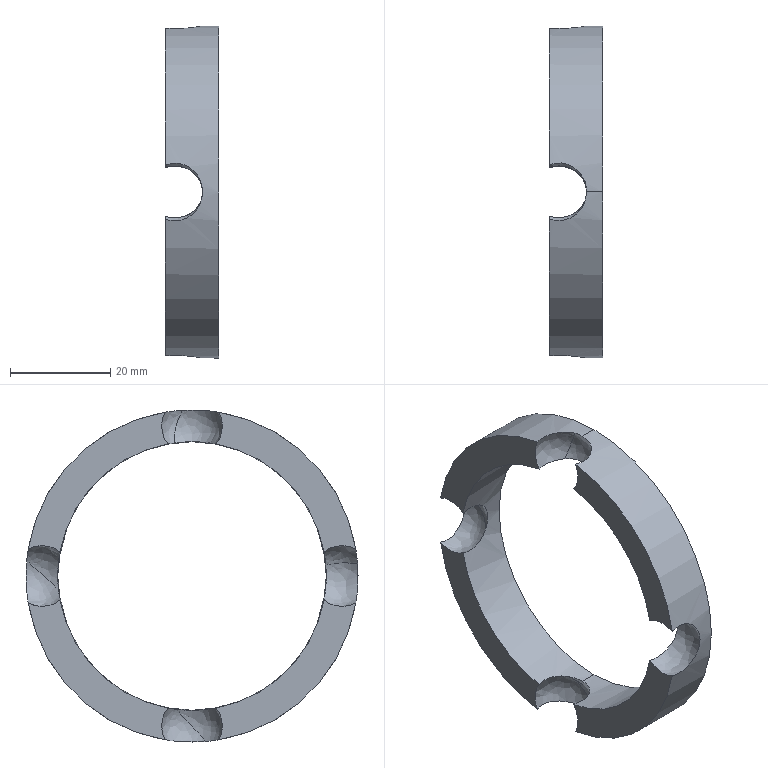Part | SolidWorks | features BaseBody 1 | 1 solid | 17 faces | volume 10638 mm3 | spline 10 | plane 5 | cylinder 2 | commonest cylinder face diameters 66.35 x2
STEP:
#1=CARTESIAN_POINT('',(4.998,48.263,51.37));
#2=VERTEX_POINT('',#1);
#3=CARTESIAN_POINT('',(-1.905,48.619,54.059));
#4=VERTEX_POINT('',#3);
#5=CARTESIAN_POINT('',(4.998,48.263,51.37));
#6=CARTESIAN_POINT('',(4.85,48.288,51.674));
#7=CARTESIAN_POINT('',(4.671,48.316,51.963));
#8=CARTESIAN_POINT('',(4.265,48.377,52.495));
#9=CARTESIAN_POINT('',(4.034,48.409,52.744));
#10=CARTESIAN_POINT('',(3.53,48.473,53.191));
#11=CARTESIAN_POINT('',(3.259,48.504,53.389));
#12=CARTESIAN_POINT('',(2.684,48.561,53.735));
#13=CARTESIAN_POINT('',(2.377,48.587,53.884));
#14=CARTESIAN_POINT('',(1.748,48.63,54.121));
#15=CARTESIAN_POINT('',(1.425,48.647,54.212));
#16=CARTESIAN_POINT('',(0.7618,48.671,54.337));
#17=CARTESIAN_POINT('',(0.4216,48.678,54.371));
#18=CARTESIAN_POINT('',(-0.5983,48.681,54.386));
#19=CARTESIAN_POINT('',(-1.263,48.66,54.281));
#20=CARTESIAN_POINT('',(-1.905,48.619,54.059));
#21=B_SPLINE_CURVE_WITH_KNOTS('',3,(#5,#6,#7,#8,#9,#10,#11,#12,#13,#14,#15,#16,#17,#18,#19,#20),.UNSPECIFIED.,.F.,.F.,(4,2,2,2,2,2,2,4),(0.01061,0.01162,0.01262,0.01363,0.01463,0.01564,0.01665,0.01866),.UNSPECIFIED.);
#22=EDGE_CURVE('',#2,#4,#21,.T.);
#23=ORIENTED_EDGE('',*,*,#22,.F.);
#24=CARTESIAN_POINT('',(5.424,47.273,51.598));
#25=VERTEX_POINT('',#24);
#26=CARTESIAN_POINT('',(0.,45.,49.2));
#27=DIRECTION('',(0.4147,-0.03029,-0.9094));
#28=DIRECTION('',(-0.854,-0.3579,-0.3775));
#29=AXIS2_PLACEMENT_3D('',#26,#27,#28);
#30=CIRCLE('',#29,6.351);
#31=EDGE_CURVE('',#2,#25,#30,.T.);
#32=ORIENTED_EDGE('',*,*,#31,.T.);
#33=CARTESIAN_POINT('',(5.009,41.911,51.587));
#34=VERTEX_POINT('',#33);
#35=CARTESIAN_POINT('',(0.,45.,49.2));
#36=DIRECTION('',(-0.4147,0.03029,0.9094));
#37=DIRECTION('',(-0.854,-0.3579,-0.3775));
#38=AXIS2_PLACEMENT_3D('',#35,#36,#37);
#39=CIRCLE('',#38,6.351);
#40=EDGE_CURVE('',#34,#25,#39,.T.);
#41=ORIENTED_EDGE('',*,*,#40,.F.);
#42=CARTESIAN_POINT('',(-1.905,42.269,54.608));
#43=VERTEX_POINT('',#42);
#44=CARTESIAN_POINT('',(-1.905,42.269,54.608));
#45=CARTESIAN_POINT('',(-1.577,42.29,54.734));
#46=CARTESIAN_POINT('',(-1.243,42.305,54.826));
#47=CARTESIAN_POINT('',(-0.7316,42.321,54.914));
#48=CARTESIAN_POINT('',(-0.5596,42.325,54.935));
#49=CARTESIAN_POINT('',(-0.2125,42.329,54.961));
#50=CARTESIAN_POINT('',(-0.03628,42.33,54.965));
#51=CARTESIAN_POINT('',(0.4893,42.327,54.951));
#52=CARTESIAN_POINT('',(0.8336,42.32,54.908));
#53=CARTESIAN_POINT('',(1.511,42.293,54.754));
#54=CARTESIAN_POINT('',(1.847,42.274,54.642));
#55=CARTESIAN_POINT('',(2.481,42.228,54.359));
#56=CARTESIAN_POINT('',(2.782,42.202,54.188));
#57=CARTESIAN_POINT('',(3.21,42.158,53.889));
#58=CARTESIAN_POINT('',(3.349,42.143,53.781));
#59=CARTESIAN_POINT('',(3.614,42.112,53.555));
#60=CARTESIAN_POINT('',(3.74,42.096,53.436));
#61=CARTESIAN_POINT('',(4.102,42.05,53.064));
#62=CARTESIAN_POINT('',(4.319,42.019,52.794));
#63=CARTESIAN_POINT('',(4.707,41.961,52.211));
#64=CARTESIAN_POINT('',(4.872,41.934,51.905));
#65=CARTESIAN_POINT('',(5.009,41.911,51.587));
#66=B_SPLINE_CURVE_WITH_KNOTS('',3,(#44,#45,#46,#47,#48,#49,#50,#51,#52,#53,#54,#55,#56,#57,#58,#59,#60,#61,#62,#63,#64,#65),.UNSPECIFIED.,.F.,.F.,(4,2,2,2,2,2,2,2,2,2,4),(-0.01955,-0.01851,-0.01799,-0.01747,-0.01643,-0.0154,-0.01436,-0.01384,-0.01332,-0.01228,-0.01124),.UNSPECIFIED.);
#67=EDGE_CURVE('',#43,#34,#66,.T.);
#68=ORIENTED_EDGE('',*,*,#67,.F.);
#69=CARTESIAN_POINT('',(-1.905,45.,49.2));
#70=DIRECTION('',(1.,0.,0.));
#71=DIRECTION('',(0.,0.,-1.));
#72=AXIS2_PLACEMENT_3D('',#69,#70,#71);
#73=CIRCLE('',#72,6.059);
#74=EDGE_CURVE('',#4,#43,#73,.T.);
#75=ORIENTED_EDGE('',*,*,#74,.F.);
#76=EDGE_LOOP('',(#23,#32,#41,#68,#75));
#77=FACE_OUTER_BOUND('',#76,.T.);
#78=CARTESIAN_POINT('',(-2.519,50.674,47.862));
#79=CARTESIAN_POINT('',(-7.762,51.057,59.358));
#80=CARTESIAN_POINT('',(-3.792,39.261,61.561));
#81=CARTESIAN_POINT('',(1.451,38.878,50.065));
#82=CARTESIAN_POINT('',(0.7712,52.475,49.303));
#83=CARTESIAN_POINT('',(-4.799,52.882,61.518));
#84=CARTESIAN_POINT('',(-0.5807,40.346,63.86));
#85=CARTESIAN_POINT('',(4.99,39.939,51.644));
#86=CARTESIAN_POINT('',(4.162,51.023,50.897));
#87=CARTESIAN_POINT('',(0.8289,51.267,58.206));
#88=CARTESIAN_POINT('',(3.353,43.767,59.607));
#89=CARTESIAN_POINT('',(6.686,43.523,52.298));
#90=CARTESIAN_POINT('',(5.424,47.273,51.598));
#91=CARTESIAN_POINT('',(5.424,47.273,51.598));
#92=CARTESIAN_POINT('',(5.424,47.273,51.598));
#93=CARTESIAN_POINT('',(5.424,47.273,51.598));
#94=(BOUNDED_SURFACE()B_SPLINE_SURFACE(3,3,((#78,#79,#80,#81),(#82,#83,#84,#85),(#86,#87,#88,#89),(#90,#91,#92,#93)),.UNSPECIFIED.,.F.,.F.,.F.)B_SPLINE_SURFACE_WITH_KNOTS((4,4),(4,4),(0.,1.),(0.,1.),.UNSPECIFIED.)GEOMETRIC_REPRESENTATION_ITEM()RATIONAL_B_SPLINE_SURFACE(((1.,0.3333,0.3333,1.),(0.7809,0.2603,0.2603,0.7809),(0.7809,0.2603,0.2603,0.7809),(1.,0.3333,0.3333,1.)))REPRESENTATION_ITEM('')SURFACE());
#95=ADVANCED_FACE('',(#77),#94,.T.);
#96=CARTESIAN_POINT('',(4.024,78.538,75.791));
#97=VERTEX_POINT('',#96);
#98=CARTESIAN_POINT('',(-1.905,79.859,75.581));
#99=VERTEX_POINT('',#98);
#100=CARTESIAN_POINT('',(4.024,78.538,75.791));
#101=CARTESIAN_POINT('',(3.838,78.726,75.766));
#102=CARTESIAN_POINT('',(3.637,78.9,75.741));
#103=CARTESIAN_POINT('',(3.21,79.218,75.692));
#104=CARTESIAN_POINT('',(2.983,79.363,75.668));
#105=CARTESIAN_POINT('',(2.515,79.615,75.625));
#106=CARTESIAN_POINT('',(2.273,79.724,75.606));
#107=CARTESIAN_POINT('',(1.774,79.909,75.572));
#108=CARTESIAN_POINT('',(1.515,79.985,75.558));
#109=CARTESIAN_POINT('',(0.9921,80.099,75.536));
#110=CARTESIAN_POINT('',(0.7281,80.138,75.528));
#111=CARTESIAN_POINT('',(0.1951,80.18,75.52));
#112=CARTESIAN_POINT('',(-0.07553,80.182,75.52));
#113=CARTESIAN_POINT('',(-0.8755,80.136,75.529));
#114=CARTESIAN_POINT('',(-1.397,80.034,75.549));
#115=CARTESIAN_POINT('',(-1.905,79.859,75.581));
#116=B_SPLINE_CURVE_WITH_KNOTS('',3,(#100,#101,#102,#103,#104,#105,#106,#107,#108,#109,#110,#111,#112,#113,#114,#115),.UNSPECIFIED.,.F.,.F.,(4,2,2,2,2,2,2,4),(0.00392,0.004717,0.005515,0.006312,0.007109,0.007906,0.008703,0.0103),.UNSPECIFIED.);
#117=EDGE_CURVE('',#97,#99,#116,.T.);
#118=ORIENTED_EDGE('',*,*,#117,.F.);
#119=CARTESIAN_POINT('',(5.424,77.273,81.598));
#120=VERTEX_POINT('',#119);
#121=CARTESIAN_POINT('',(0.,75.,79.2));
#122=DIRECTION('',(0.4774,-0.8276,-0.2953));
#123=DIRECTION('',(-0.854,-0.3579,-0.3775));
#124=AXIS2_PLACEMENT_3D('',#121,#122,#123);
#125=CIRCLE('',#124,6.351);
#126=EDGE_CURVE('',#97,#120,#125,.T.);
#127=ORIENTED_EDGE('',*,*,#126,.T.);
#128=CARTESIAN_POINT('',(5.2,76.886,82.321));
#129=VERTEX_POINT('',#128);
#130=CARTESIAN_POINT('',(0.,75.,79.2));
#131=DIRECTION('',(-0.4774,0.8276,0.2953));
#132=DIRECTION('',(-0.854,-0.3579,-0.3775));
#133=AXIS2_PLACEMENT_3D('',#130,#131,#132);
#134=CIRCLE('',#133,6.351);
#135=EDGE_CURVE('',#129,#120,#134,.T.);
#136=ORIENTED_EDGE('',*,*,#135,.F.);
#137=CARTESIAN_POINT('',(-1.905,80.408,81.931));
#138=VERTEX_POINT('',#137);
#139=CARTESIAN_POINT('',(-1.905,80.408,81.931));
#140=CARTESIAN_POINT('',(-1.556,80.542,81.909));
#141=CARTESIAN_POINT('',(-1.2,80.638,81.893));
#142=CARTESIAN_POINT('',(-0.6542,80.725,81.877));
#143=CARTESIAN_POINT('',(-0.4706,80.744,81.874));
#144=CARTESIAN_POINT('',(-0.09979,80.764,81.87));
#145=CARTESIAN_POINT('',(0.08844,80.765,81.87));
#146=CARTESIAN_POINT('',(0.6454,80.736,81.875));
#147=CARTESIAN_POINT('',(1.01,80.678,81.886));
#148=CARTESIAN_POINT('',(1.726,80.487,81.918));
#149=CARTESIAN_POINT('',(2.077,80.352,81.941));
#150=CARTESIAN_POINT('',(2.735,80.019,81.994));
#151=CARTESIAN_POINT('',(3.046,79.819,82.024));
#152=CARTESIAN_POINT('',(3.629,79.354,82.089));
#153=CARTESIAN_POINT('',(3.892,79.096,82.122));
#154=CARTESIAN_POINT('',(4.367,78.532,82.188));
#155=CARTESIAN_POINT('',(4.579,78.223,82.22));
#156=CARTESIAN_POINT('',(4.937,77.576,82.276));
#157=CARTESIAN_POINT('',(5.084,77.238,82.301));
#158=CARTESIAN_POINT('',(5.2,76.886,82.321));
#159=B_SPLINE_CURVE_WITH_KNOTS('',3,(#139,#140,#141,#142,#143,#144,#145,#146,#147,#148,#149,#150,#151,#152,#153,#154,#155,#156,#157,#158),.UNSPECIFIED.,.F.,.F.,(4,2,2,2,2,2,2,2,2,4),(-0.01954,-0.01843,-0.01788,-0.01733,-0.01622,-0.01512,-0.01402,-0.01291,-0.01181,-0.0107),.UNSPECIFIED.);
#160=EDGE_CURVE('',#138,#129,#159,.T.);
#161=ORIENTED_EDGE('',*,*,#160,.F.);
#162=CARTESIAN_POINT('',(-1.905,75.,79.2));
#163=DIRECTION('',(1.,0.,0.));
#164=DIRECTION('',(0.,0.,-1.));
#165=AXIS2_PLACEMENT_3D('',#162,#163,#164);
#166=CIRCLE('',#165,6.059);
#167=EDGE_CURVE('',#99,#138,#166,.T.);
#168=ORIENTED_EDGE('',*,*,#167,.F.);
#169=EDGE_LOOP('',(#118,#127,#136,#161,#168));
#170=FACE_OUTER_BOUND('',#169,.T.);
#171=CARTESIAN_POINT('',(0.1572,77.214,73.249));
#172=CARTESIAN_POINT('',(-5.774,87.496,76.918));
#173=CARTESIAN_POINT('',(-8.343,82.124,87.823));
#174=CARTESIAN_POINT('',(-2.412,71.841,84.154));
#175=CARTESIAN_POINT('',(3.996,79.137,74.066));
#176=CARTESIAN_POINT('',(-2.803,90.923,78.271));
#177=CARTESIAN_POINT('',(-5.747,84.765,90.77));
#178=CARTESIAN_POINT('',(1.051,72.979,86.565));
#179=CARTESIAN_POINT('',(6.327,79.163,77.762));
#180=CARTESIAN_POINT('',(2.155,86.396,80.343));
#181=CARTESIAN_POINT('',(0.3478,82.617,88.014));
#182=CARTESIAN_POINT('',(4.52,75.384,85.433));
#183=CARTESIAN_POINT('',(5.424,77.273,81.598));
#184=CARTESIAN_POINT('',(5.424,77.273,81.598));
#185=CARTESIAN_POINT('',(5.424,77.273,81.598));
#186=CARTESIAN_POINT('',(5.424,77.273,81.598));
#187=(BOUNDED_SURFACE()B_SPLINE_SURFACE(3,3,((#171,#172,#173,#174),(#175,#176,#177,#178),(#179,#180,#181,#182),(#183,#184,#185,#186)),.UNSPECIFIED.,.F.,.F.,.T.)B_SPLINE_SURFACE_WITH_KNOTS((4,4),(4,4),(0.,1.),(0.,1.),.UNSPECIFIED.)GEOMETRIC_REPRESENTATION_ITEM()RATIONAL_B_SPLINE_SURFACE(((1.,0.3333,0.3333,1.),(0.7529,0.251,0.251,0.7529),(0.7529,0.251,0.251,0.7529),(1.,0.3333,0.3333,1.)))REPRESENTATION_ITEM('')SURFACE());
#188=ADVANCED_FACE('',(#170),#187,.T.);
#189=CARTESIAN_POINT('',(4.675,101.685,46.463));
#190=VERTEX_POINT('',#189);
#191=CARTESIAN_POINT('',(-1.905,101.381,44.341));
#192=VERTEX_POINT('',#191);
#193=CARTESIAN_POINT('',(4.675,101.685,46.463));
#194=CARTESIAN_POINT('',(4.505,101.659,46.205));
#195=CARTESIAN_POINT('',(4.314,101.63,45.964));
#196=CARTESIAN_POINT('',(3.887,101.572,45.516));
#197=CARTESIAN_POINT('',(3.652,101.542,45.309));
#198=CARTESIAN_POINT('',(3.156,101.486,44.943));
#199=CARTESIAN_POINT('',(2.894,101.459,44.782));
#200=CARTESIAN_POINT('',(2.339,101.411,44.501));
#201=CARTESIAN_POINT('',(2.05,101.389,44.384));
#202=CARTESIAN_POINT('',(1.462,101.355,44.199));
#203=CARTESIAN_POINT('',(1.16,101.342,44.13));
#204=CARTESIAN_POINT('',(0.5433,101.324,44.04));
#205=CARTESIAN_POINT('',(0.2296,101.32,44.019));
#206=CARTESIAN_POINT('',(-0.7067,101.323,44.033));
#207=CARTESIAN_POINT('',(-1.314,101.344,44.137));
#208=CARTESIAN_POINT('',(-1.905,101.381,44.341));
#209=B_SPLINE_CURVE_WITH_KNOTS('',3,(#193,#194,#195,#196,#197,#198,#199,#200,#201,#202,#203,#204,#205,#206,#207,#208),.UNSPECIFIED.,.F.,.F.,(4,2,2,2,2,2,2,4),(0.01126,0.01218,0.01311,0.01403,0.01496,0.01588,0.01681,0.01866),.UNSPECIFIED.);
#210=EDGE_CURVE('',#190,#192,#209,.T.);
#211=ORIENTED_EDGE('',*,*,#210,.F.);
#212=CARTESIAN_POINT('',(5.424,107.273,51.598));
#213=VERTEX_POINT('',#212);
#214=CARTESIAN_POINT('',(0.,105.,49.2));
#215=DIRECTION('',(-0.0446,-0.6727,0.7386));
#216=DIRECTION('',(-0.854,-0.3579,-0.3775));
#217=AXIS2_PLACEMENT_3D('',#214,#215,#216);
#218=CIRCLE('',#217,6.351);
#219=EDGE_CURVE('',#190,#213,#218,.T.);
#220=ORIENTED_EDGE('',*,*,#219,.T.);
#221=CARTESIAN_POINT('',(4.674,108.035,52.246));
#222=VERTEX_POINT('',#221);
#223=CARTESIAN_POINT('',(0.,105.,49.2));
#224=DIRECTION('',(0.0446,0.6727,-0.7386));
#225=DIRECTION('',(-0.854,-0.3579,-0.3775));
#226=AXIS2_PLACEMENT_3D('',#223,#224,#225);
#227=CIRCLE('',#226,6.351);
#228=EDGE_CURVE('',#222,#213,#227,.T.);
#229=ORIENTED_EDGE('',*,*,#228,.F.);
#230=CARTESIAN_POINT('',(-1.905,107.731,43.792));
#231=VERTEX_POINT('',#230);
#232=CARTESIAN_POINT('',(-1.905,107.731,43.792));
#233=CARTESIAN_POINT('',(-1.355,107.696,43.581));
#234=CARTESIAN_POINT('',(-0.7877,107.675,43.464));
#235=CARTESIAN_POINT('',(0.09096,107.669,43.431));
#236=CARTESIAN_POINT('',(0.3863,107.672,43.444));
#237=CARTESIAN_POINT('',(0.9633,107.685,43.518));
#238=CARTESIAN_POINT('',(1.248,107.695,43.579));
#239=CARTESIAN_POINT('',(1.808,107.724,43.747));
#240=CARTESIAN_POINT('',(2.083,107.742,43.856));
#241=CARTESIAN_POINT('',(2.605,107.783,44.111));
#242=CARTESIAN_POINT('',(2.854,107.806,44.26));
#243=CARTESIAN_POINT('',(3.33,107.855,44.597));
#244=CARTESIAN_POINT('',(3.556,107.881,44.787));
#245=CARTESIAN_POINT('',(3.97,107.933,45.193));
#246=CARTESIAN_POINT('',(4.161,107.959,45.412));
#247=CARTESIAN_POINT('',(4.509,108.009,45.879));
#248=CARTESIAN_POINT('',(4.667,108.033,46.128));
#249=CARTESIAN_POINT('',(4.94,108.077,46.642));
#250=CARTESIAN_POINT('',(5.057,108.097,46.907));
#251=CARTESIAN_POINT('',(5.252,108.13,47.456));
#252=CARTESIAN_POINT('',(5.33,108.144,47.742));
#253=CARTESIAN_POINT('',(5.443,108.164,48.315));
#254=CARTESIAN_POINT('',(5.478,108.171,48.603));
#255=CARTESIAN_POINT('',(5.507,108.176,49.184));
#256=CARTESIAN_POINT('',(5.501,108.175,49.478));
#257=CARTESIAN_POINT('',(5.446,108.165,50.063));
#258=CARTESIAN_POINT('',(5.398,108.156,50.35));
#259=CARTESIAN_POINT('',(5.261,108.132,50.914));
#260=CARTESIAN_POINT('',(5.172,108.116,51.191));
#261=CARTESIAN_POINT('',(4.952,108.079,51.734));
#262=CARTESIAN_POINT('',(4.822,108.058,51.997));
#263=CARTESIAN_POINT('',(4.674,108.035,52.246));
#264=B_SPLINE_CURVE_WITH_KNOTS('',3,(#232,#233,#234,#235,#236,#237,#238,#239,#240,#241,#242,#243,#244,#245,#246,#247,#248,#249,#250,#251,#252,#253,#254,#255,#256,#257,#258,#259,#260,#261,#262,#263),.UNSPECIFIED.,.F.,.F.,(4,2,2,2,2,2,2,2,2,2,2,2,2,2,2,4),(0.,0.001739,0.002609,0.003479,0.004349,0.005218,0.006088,0.006958,0.007827,0.008697,0.009567,0.01044,0.01131,0.01218,0.01305,0.01392),.UNSPECIFIED.);
#265=EDGE_CURVE('',#231,#222,#264,.T.);
#266=ORIENTED_EDGE('',*,*,#265,.F.);
#267=CARTESIAN_POINT('',(-1.905,105.,49.2));
#268=DIRECTION('',(1.,0.,0.));
#269=DIRECTION('',(0.,0.,-1.));
#270=AXIS2_PLACEMENT_3D('',#267,#268,#269);
#271=CIRCLE('',#270,6.059);
#272=EDGE_CURVE('',#192,#231,#271,.T.);
#273=ORIENTED_EDGE('',*,*,#272,.F.);
#274=EDGE_LOOP('',(#211,#220,#229,#266,#273));
#275=FACE_OUTER_BOUND('',#274,.T.);
#276=CARTESIAN_POINT('',(-1.969,100.595,45.07));
#277=CARTESIAN_POINT('',(-1.6,106.163,38.956));
#278=CARTESIAN_POINT('',(-5.89,111.524,43.579));
#279=CARTESIAN_POINT('',(-6.259,105.956,49.693));
#280=CARTESIAN_POINT('',(4.705,98.783,43.822));
#281=CARTESIAN_POINT('',(5.549,111.521,29.835));
#282=CARTESIAN_POINT('',(-4.266,123.785,40.411));
#283=CARTESIAN_POINT('',(-5.111,111.047,54.398));
#284=CARTESIAN_POINT('',(9.066,102.722,47.673));
#285=CARTESIAN_POINT('',(9.693,112.176,37.293));
#286=CARTESIAN_POINT('',(2.409,121.277,45.142));
#287=CARTESIAN_POINT('',(1.782,111.824,55.522));
#288=CARTESIAN_POINT('',(5.424,107.273,51.598));
#289=CARTESIAN_POINT('',(5.424,107.273,51.598));
#290=CARTESIAN_POINT('',(5.424,107.273,51.598));
#291=CARTESIAN_POINT('',(5.424,107.273,51.598));
#292=(BOUNDED_SURFACE()B_SPLINE_SURFACE(3,3,((#276,#277,#278,#279),(#280,#281,#282,#283),(#284,#285,#286,#287),(#288,#289,#290,#291)),.UNSPECIFIED.,.F.,.F.,.F.)B_SPLINE_SURFACE_WITH_KNOTS((4,4),(4,4),(0.,1.),(0.,1.),.UNSPECIFIED.)GEOMETRIC_REPRESENTATION_ITEM()RATIONAL_B_SPLINE_SURFACE(((1.,0.3333,0.3333,1.),(0.565,0.1883,0.1883,0.565),(0.565,0.1883,0.1883,0.565),(1.,0.3333,0.3333,1.)))REPRESENTATION_ITEM('')SURFACE());
#293=ADVANCED_FACE('',(#275),#292,.T.);
#294=CARTESIAN_POINT('',(4.358,78.168,22.563));
#295=VERTEX_POINT('',#294);
#296=CARTESIAN_POINT('',(5.5,75.,22.375));
#297=VERTEX_POINT('',#296);
#298=CARTESIAN_POINT('',(4.358,78.168,22.563));
#299=CARTESIAN_POINT('',(4.537,77.949,22.537));
#300=CARTESIAN_POINT('',(4.7,77.713,22.511));
#301=CARTESIAN_POINT('',(4.985,77.214,22.465));
#302=CARTESIAN_POINT('',(5.105,76.956,22.445));
#303=CARTESIAN_POINT('',(5.396,76.155,22.395));
#304=CARTESIAN_POINT('',(5.5,75.579,22.375));
#305=CARTESIAN_POINT('',(5.5,75.,22.375));
#306=B_SPLINE_CURVE_WITH_KNOTS('',3,(#298,#299,#300,#301,#302,#303,#304,#305),.UNSPECIFIED.,.F.,.F.,(4,2,2,4),(0.004949,0.005803,0.006658,0.008367),.UNSPECIFIED.);
#307=EDGE_CURVE('',#295,#297,#306,.T.);
#308=ORIENTED_EDGE('',*,*,#307,.F.);
#309=CARTESIAN_POINT('',(5.424,77.273,21.598));
#310=VERTEX_POINT('',#309);
#311=CARTESIAN_POINT('',(0.,75.,19.2));
#312=DIRECTION('',(-0.004434,0.7307,-0.6827));
#313=DIRECTION('',(-0.854,-0.3579,-0.3775));
#314=AXIS2_PLACEMENT_3D('',#311,#312,#313);
#315=CIRCLE('',#314,6.351);
#316=EDGE_CURVE('',#295,#310,#315,.T.);
#317=ORIENTED_EDGE('',*,*,#316,.T.);
#318=CARTESIAN_POINT('',(4.798,72.175,16.145));
#319=VERTEX_POINT('',#318);
#320=CARTESIAN_POINT('',(0.,75.,19.2));
#321=DIRECTION('',(0.004434,-0.7307,0.6827));
#322=DIRECTION('',(-0.854,-0.3579,-0.3775));
#323=AXIS2_PLACEMENT_3D('',#320,#321,#322);
#324=CIRCLE('',#323,6.351);
#325=EDGE_CURVE('',#319,#310,#324,.T.);
#326=ORIENTED_EDGE('',*,*,#325,.F.);
#327=CARTESIAN_POINT('',(-1.905,69.592,16.469));
#328=VERTEX_POINT('',#327);
#329=CARTESIAN_POINT('',(-1.905,69.592,16.469));
#330=CARTESIAN_POINT('',(-1.288,69.355,16.508));
#331=CARTESIAN_POINT('',(-0.6467,69.236,16.53));
#332=CARTESIAN_POINT('',(0.347,69.239,16.529));
#333=CARTESIAN_POINT('',(0.6729,69.271,16.523));
#334=CARTESIAN_POINT('',(1.314,69.393,16.502));
#335=CARTESIAN_POINT('',(1.632,69.485,16.486));
#336=CARTESIAN_POINT('',(2.245,69.725,16.447));
#337=CARTESIAN_POINT('',(2.536,69.872,16.423));
#338=CARTESIAN_POINT('',(3.091,70.216,16.371));
#339=CARTESIAN_POINT('',(3.356,70.416,16.343));
#340=CARTESIAN_POINT('',(3.841,70.854,16.284));
#341=CARTESIAN_POINT('',(4.062,71.093,16.255));
#342=CARTESIAN_POINT('',(4.464,71.608,16.198));
#343=CARTESIAN_POINT('',(4.645,71.887,16.17));
#344=CARTESIAN_POINT('',(4.798,72.175,16.145));
#345=B_SPLINE_CURVE_WITH_KNOTS('',3,(#329,#330,#331,#332,#333,#334,#335,#336,#337,#338,#339,#340,#341,#342,#343,#344),.UNSPECIFIED.,.F.,.F.,(4,2,2,2,2,2,2,4),(-0.001944,0.00001557,0.0009952,0.001975,0.002955,0.003934,0.004914,0.005894),.UNSPECIFIED.);
#346=EDGE_CURVE('',#328,#319,#345,.T.);
#347=ORIENTED_EDGE('',*,*,#346,.F.);
#348=CARTESIAN_POINT('',(-1.905,70.141,22.819));
#349=VERTEX_POINT('',#348);
#350=CARTESIAN_POINT('',(-1.905,75.,19.2));
#351=DIRECTION('',(1.,0.,0.));
#352=DIRECTION('',(0.,0.,-1.));
#353=AXIS2_PLACEMENT_3D('',#350,#351,#352);
#354=CIRCLE('',#353,6.059);
#355=EDGE_CURVE('',#349,#328,#354,.T.);
#356=ORIENTED_EDGE('',*,*,#355,.F.);
#357=CARTESIAN_POINT('',(5.5,75.,22.375));
#358=CARTESIAN_POINT('',(5.5,74.564,22.375));
#359=CARTESIAN_POINT('',(5.443,74.139,22.386));
#360=CARTESIAN_POINT('',(5.276,73.515,22.415));
#361=CARTESIAN_POINT('',(5.206,73.308,22.428));
#362=CARTESIAN_POINT('',(5.041,72.91,22.456));
#363=CARTESIAN_POINT('',(4.947,72.718,22.472));
#364=CARTESIAN_POINT('',(4.627,72.16,22.523));
#365=CARTESIAN_POINT('',(4.364,71.811,22.563));
#366=CARTESIAN_POINT('',(3.916,71.35,22.624));
#367=CARTESIAN_POINT('',(3.758,71.206,22.644));
#368=CARTESIAN_POINT('',(3.425,70.936,22.684));
#369=CARTESIAN_POINT('',(3.249,70.811,22.704));
#370=CARTESIAN_POINT('',(2.7,70.466,22.76));
#371=CARTESIAN_POINT('',(2.313,70.282,22.793));
#372=CARTESIAN_POINT('',(1.703,70.071,22.832));
#373=CARTESIAN_POINT('',(1.493,70.012,22.843));
#374=CARTESIAN_POINT('',(1.071,69.917,22.861));
#375=CARTESIAN_POINT('',(0.8587,69.882,22.868));
#376=CARTESIAN_POINT('',(0.2161,69.811,22.882));
#377=CARTESIAN_POINT('',(-0.2224,69.812,22.881));
#378=CARTESIAN_POINT('',(-1.076,69.906,22.863));
#379=CARTESIAN_POINT('',(-1.495,69.999,22.845));
#380=CARTESIAN_POINT('',(-1.905,70.141,22.819));
#381=B_SPLINE_CURVE_WITH_KNOTS('',3,(#357,#358,#359,#360,#361,#362,#363,#364,#365,#366,#367,#368,#369,#370,#371,#372,#373,#374,#375,#376,#377,#378,#379,#380),.UNSPECIFIED.,.F.,.F.,(4,2,2,2,2,2,2,2,2,2,2,4),(0.008367,0.009653,0.0103,0.01094,0.01223,0.01287,0.01351,0.0148,0.01544,0.01608,0.01737,0.01866),.UNSPECIFIED.);
#382=EDGE_CURVE('',#297,#349,#381,.T.);
#383=ORIENTED_EDGE('',*,*,#382,.F.);
#384=EDGE_LOOP('',(#308,#317,#326,#347,#356,#383));
#385=FACE_OUTER_BOUND('',#384,.T.);
#386=CARTESIAN_POINT('',(-6.223,75.845,20.145));
#387=CARTESIAN_POINT('',(-6.185,69.532,26.042));
#388=CARTESIAN_POINT('',(-1.691,64.51,20.638));
#389=CARTESIAN_POINT('',(-1.729,70.822,14.74));
#390=CARTESIAN_POINT('',(-4.86,80.42,25.032));
#391=CARTESIAN_POINT('',(-4.778,66.788,37.769));
#392=CARTESIAN_POINT('',(4.928,55.942,26.098));
#393=CARTESIAN_POINT('',(4.845,69.574,13.361));
#394=CARTESIAN_POINT('',(1.87,81.245,25.872));
#395=CARTESIAN_POINT('',(1.93,71.261,35.201));
#396=CARTESIAN_POINT('',(9.039,63.317,26.652));
#397=CARTESIAN_POINT('',(8.978,73.301,17.323));
#398=CARTESIAN_POINT('',(5.424,77.273,21.598));
#399=CARTESIAN_POINT('',(5.424,77.273,21.598));
#400=CARTESIAN_POINT('',(5.424,77.273,21.598));
#401=CARTESIAN_POINT('',(5.424,77.273,21.598));
#402=(BOUNDED_SURFACE()B_SPLINE_SURFACE(3,3,((#386,#387,#388,#389),(#390,#391,#392,#393),(#394,#395,#396,#397),(#398,#399,#400,#401)),.UNSPECIFIED.,.F.,.F.,.F.)B_SPLINE_SURFACE_WITH_KNOTS((4,4),(4,4),(0.,1.),(0.,1.),.UNSPECIFIED.)GEOMETRIC_REPRESENTATION_ITEM()RATIONAL_B_SPLINE_SURFACE(((1.,0.3333,0.3333,1.),(0.5769,0.1923,0.1923,0.5769),(0.5769,0.1923,0.1923,0.5769),(1.,0.3333,0.3333,1.)))REPRESENTATION_ITEM('')SURFACE());
#403=ADVANCED_FACE('',(#385),#402,.T.);
#404=CARTESIAN_POINT('',(-1.905,70.141,75.581));
#405=VERTEX_POINT('',#404);
#406=CARTESIAN_POINT('',(5.5,75.,76.025));
#407=VERTEX_POINT('',#406);
#408=CARTESIAN_POINT('',(-1.905,70.141,75.581));
#409=CARTESIAN_POINT('',(-1.494,69.999,75.555));
#410=CARTESIAN_POINT('',(-1.075,69.906,75.537));
#411=CARTESIAN_POINT('',(-0.2213,69.812,75.519));
#412=CARTESIAN_POINT('',(0.2179,69.812,75.519));
#413=CARTESIAN_POINT('',(1.072,69.906,75.537));
#414=CARTESIAN_POINT('',(1.492,69.999,75.555));
#415=CARTESIAN_POINT('',(2.313,70.281,75.607));
#416=CARTESIAN_POINT('',(2.699,70.466,75.64));
#417=CARTESIAN_POINT('',(3.425,70.921,75.714));
#418=CARTESIAN_POINT('',(3.766,71.195,75.756));
#419=CARTESIAN_POINT('',(4.361,71.808,75.836));
#420=CARTESIAN_POINT('',(4.621,72.151,75.876));
#421=CARTESIAN_POINT('',(5.053,72.902,75.945));
#422=CARTESIAN_POINT('',(5.217,73.297,75.974));
#423=CARTESIAN_POINT('',(5.385,73.921,76.004));
#424=CARTESIAN_POINT('',(5.429,74.135,76.012));
#425=CARTESIAN_POINT('',(5.486,74.565,76.022));
#426=CARTESIAN_POINT('',(5.5,74.782,76.025));
#427=CARTESIAN_POINT('',(5.5,75.,76.025));
#428=B_SPLINE_CURVE_WITH_KNOTS('',3,(#408,#409,#410,#411,#412,#413,#414,#415,#416,#417,#418,#419,#420,#421,#422,#423,#424,#425,#426,#427),.UNSPECIFIED.,.F.,.F.,(4,2,2,2,2,2,2,2,2,4),(-0.01031,-0.009019,-0.00773,-0.006442,-0.005154,-0.003865,-0.002577,-0.001288,-0.0006442,0.),.UNSPECIFIED.);
#429=EDGE_CURVE('',#405,#407,#428,.T.);
#430=ORIENTED_EDGE('',*,*,#429,.T.);
#431=CARTESIAN_POINT('',(8.7,75.,76.025));
#432=VERTEX_POINT('',#431);
#433=CARTESIAN_POINT('',(3.397,75.,76.025));
#434=DIRECTION('',(1.,0.,0.));
#435=VECTOR('',#434,1000.);
#436=LINE('',#433,#435);
#437=EDGE_CURVE('',#407,#432,#436,.T.);
#438=ORIENTED_EDGE('',*,*,#437,.T.);
#439=CARTESIAN_POINT('',(8.7,75.,22.375));
#440=VERTEX_POINT('',#439);
#441=CARTESIAN_POINT('',(8.7,75.,49.2));
#442=DIRECTION('',(-1.,0.,0.));
#443=DIRECTION('',(0.,0.,-1.));
#444=AXIS2_PLACEMENT_3D('',#441,#442,#443);
#445=CIRCLE('',#444,26.825);
#446=EDGE_CURVE('',#440,#432,#445,.T.);
#447=ORIENTED_EDGE('',*,*,#446,.F.);
#448=CARTESIAN_POINT('',(3.398,75.,22.375));
#449=DIRECTION('',(1.,0.,0.));
#450=VECTOR('',#449,1000.);
#451=LINE('',#448,#450);
#452=EDGE_CURVE('',#297,#440,#451,.T.);
#453=ORIENTED_EDGE('',*,*,#452,.F.);
#454=ORIENTED_EDGE('',*,*,#382,.T.);
#455=CARTESIAN_POINT('',(-1.905,48.619,44.341));
#456=VERTEX_POINT('',#455);
#457=CARTESIAN_POINT('',(-1.905,75.,49.2));
#458=DIRECTION('',(1.,0.,0.));
#459=DIRECTION('',(0.,0.,-1.));
#460=AXIS2_PLACEMENT_3D('',#457,#458,#459);
#461=CIRCLE('',#460,26.825);
#462=EDGE_CURVE('',#456,#349,#461,.T.);
#463=ORIENTED_EDGE('',*,*,#462,.F.);
#464=CARTESIAN_POINT('',(-1.905,48.619,44.341));
#465=CARTESIAN_POINT('',(-1.405,48.651,44.168));
#466=CARTESIAN_POINT('',(-0.8924,48.671,44.068));
#467=CARTESIAN_POINT('',(-0.106,48.68,44.018));
#468=CARTESIAN_POINT('',(0.1604,48.68,44.02));
#469=CARTESIAN_POINT('',(0.6839,48.673,44.057));
#470=CARTESIAN_POINT('',(0.9427,48.666,44.093));
#471=CARTESIAN_POINT('',(1.454,48.645,44.2));
#472=CARTESIAN_POINT('',(1.708,48.632,44.271));
#473=CARTESIAN_POINT('',(2.206,48.599,44.447));
#474=CARTESIAN_POINT('',(2.445,48.58,44.552));
#475=CARTESIAN_POINT('',(2.907,48.539,44.793));
#476=CARTESIAN_POINT('',(3.129,48.517,44.929));
#477=CARTESIAN_POINT('',(3.555,48.469,45.234));
#478=CARTESIAN_POINT('',(3.759,48.444,45.404));
#479=CARTESIAN_POINT('',(4.134,48.395,45.766));
#480=CARTESIAN_POINT('',(4.307,48.371,45.96));
#481=CARTESIAN_POINT('',(4.623,48.323,46.374));
#482=CARTESIAN_POINT('',(4.768,48.301,46.596));
#483=CARTESIAN_POINT('',(5.145,48.239,47.289));
#484=CARTESIAN_POINT('',(5.321,48.208,47.779));
#485=CARTESIAN_POINT('',(5.514,48.173,48.823));
#486=CARTESIAN_POINT('',(5.527,48.17,49.346));
#487=CARTESIAN_POINT('',(5.419,48.19,50.132));
#488=CARTESIAN_POINT('',(5.362,48.2,50.39));
#489=CARTESIAN_POINT('',(5.209,48.227,50.89));
#490=CARTESIAN_POINT('',(5.113,48.244,51.134));
#491=CARTESIAN_POINT('',(4.998,48.263,51.37));
#492=B_SPLINE_CURVE_WITH_KNOTS('',3,(#464,#465,#466,#467,#468,#469,#470,#471,#472,#473,#474,#475,#476,#477,#478,#479,#480,#481,#482,#483,#484,#485,#486,#487,#488,#489,#490,#491),.UNSPECIFIED.,.F.,.F.,(4,2,2,2,2,2,2,2,2,2,2,2,2,4),(-0.001933,-0.000365,0.0004189,0.001203,0.001987,0.002771,0.003554,0.004338,0.005122,0.005906,0.007474,0.009042,0.009826,0.01061),.UNSPECIFIED.);
#493=EDGE_CURVE('',#456,#2,#492,.T.);
#494=ORIENTED_EDGE('',*,*,#493,.T.);
#495=ORIENTED_EDGE('',*,*,#22,.T.);
#496=CARTESIAN_POINT('',(-1.905,75.,49.2));
#497=DIRECTION('',(1.,0.,0.));
#498=DIRECTION('',(0.,0.,-1.));
#499=AXIS2_PLACEMENT_3D('',#496,#497,#498);
#500=CIRCLE('',#499,26.825);
#501=EDGE_CURVE('',#405,#4,#500,.T.);
#502=ORIENTED_EDGE('',*,*,#501,.F.);
#503=EDGE_LOOP('',(#430,#438,#447,#453,#454,#463,#494,#495,#502));
#504=FACE_OUTER_BOUND('',#503,.T.);
#505=CARTESIAN_POINT('',(-1.905,75.,22.375));
#506=CARTESIAN_POINT('',(8.7,75.,22.375));
#507=CARTESIAN_POINT('',(-1.905,21.35,22.375));
#508=CARTESIAN_POINT('',(8.7,21.35,22.375));
#509=CARTESIAN_POINT('',(-1.905,21.35,76.025));
#510=CARTESIAN_POINT('',(8.7,21.35,76.025));
#511=CARTESIAN_POINT('',(-1.905,75.,76.025));
#512=CARTESIAN_POINT('',(8.7,75.,76.025));
#513=(BOUNDED_SURFACE()B_SPLINE_SURFACE(3,1,((#505,#506),(#507,#508),(#509,#510),(#511,#512)),.UNSPECIFIED.,.F.,.F.,.F.)B_SPLINE_SURFACE_WITH_KNOTS((4,4),(2,2),(0.,1.),(0.,1.),.UNSPECIFIED.)GEOMETRIC_REPRESENTATION_ITEM()RATIONAL_B_SPLINE_SURFACE(((1.,1.),(0.3333,0.3333),(0.3333,0.3333),(1.,1.)))REPRESENTATION_ITEM('')SURFACE());
#514=ADVANCED_FACE('',(#504),#513,.T.);
#515=ORIENTED_EDGE('',*,*,#160,.T.);
#516=CARTESIAN_POINT('',(5.5,75.,82.375));
#517=VERTEX_POINT('',#516);
#518=CARTESIAN_POINT('',(5.2,76.886,82.321));
#519=CARTESIAN_POINT('',(5.299,76.583,82.339));
#520=CARTESIAN_POINT('',(5.375,76.269,82.352));
#521=CARTESIAN_POINT('',(5.475,75.64,82.37));
#522=CARTESIAN_POINT('',(5.5,75.321,82.375));
#523=CARTESIAN_POINT('',(5.5,75.,82.375));
#524=B_SPLINE_CURVE_WITH_KNOTS('',3,(#518,#519,#520,#521,#522,#523),.UNSPECIFIED.,.F.,.F.,(4,2,4),(-0.0107,-0.009752,-0.008803),.UNSPECIFIED.);
#525=EDGE_CURVE('',#129,#517,#524,.T.);
#526=ORIENTED_EDGE('',*,*,#525,.T.);
#527=CARTESIAN_POINT('',(8.7,75.,82.375));
#528=VERTEX_POINT('',#527);
#529=CARTESIAN_POINT('',(3.397,75.,82.375));
#530=DIRECTION('',(1.,0.,0.));
#531=VECTOR('',#530,1000.);
#532=LINE('',#529,#531);
#533=EDGE_CURVE('',#517,#528,#532,.T.);
#534=ORIENTED_EDGE('',*,*,#533,.T.);
#535=CARTESIAN_POINT('',(8.7,75.,16.025));
#536=VERTEX_POINT('',#535);
#537=CARTESIAN_POINT('',(8.7,75.,49.2));
#538=DIRECTION('',(1.,0.,0.));
#539=DIRECTION('',(0.,0.,-1.));
#540=AXIS2_PLACEMENT_3D('',#537,#538,#539);
#541=CIRCLE('',#540,33.175);
#542=EDGE_CURVE('',#536,#528,#541,.T.);
#543=ORIENTED_EDGE('',*,*,#542,.F.);
#544=CARTESIAN_POINT('',(5.5,75.,16.025));
#545=VERTEX_POINT('',#544);
#546=CARTESIAN_POINT('',(3.398,75.,16.025));
#547=DIRECTION('',(1.,0.,0.));
#548=VECTOR('',#547,1000.);
#549=LINE('',#546,#548);
#550=EDGE_CURVE('',#545,#536,#549,.T.);
#551=ORIENTED_EDGE('',*,*,#550,.F.);
#552=CARTESIAN_POINT('',(-1.905,80.408,16.469));
#553=VERTEX_POINT('',#552);
#554=CARTESIAN_POINT('',(5.5,75.,16.025));
#555=CARTESIAN_POINT('',(5.5,75.455,16.025));
#556=CARTESIAN_POINT('',(5.45,75.901,16.034));
#557=CARTESIAN_POINT('',(5.252,76.777,16.07));
#558=CARTESIAN_POINT('',(5.101,77.21,16.096));
#559=CARTESIAN_POINT('',(4.712,78.016,16.16));
#560=CARTESIAN_POINT('',(4.472,78.395,16.197));
#561=CARTESIAN_POINT('',(3.9,79.097,16.277));
#562=CARTESIAN_POINT('',(3.579,79.407,16.318));
#563=CARTESIAN_POINT('',(3.043,79.812,16.375));
#564=CARTESIAN_POINT('',(2.854,79.937,16.394));
#565=CARTESIAN_POINT('',(2.461,80.162,16.429));
#566=CARTESIAN_POINT('',(2.26,80.262,16.445));
#567=CARTESIAN_POINT('',(1.847,80.435,16.473));
#568=CARTESIAN_POINT('',(1.636,80.508,16.485));
#569=CARTESIAN_POINT('',(1.202,80.629,16.506));
#570=CARTESIAN_POINT('',(0.9791,80.676,16.514));
#571=CARTESIAN_POINT('',(0.3055,80.773,16.531));
#572=CARTESIAN_POINT('',(-0.1542,80.779,16.532));
#573=CARTESIAN_POINT('',(-1.046,80.677,16.514));
#574=CARTESIAN_POINT('',(-1.481,80.571,16.496));
#575=CARTESIAN_POINT('',(-1.905,80.408,16.469));
#576=B_SPLINE_CURVE_WITH_KNOTS('',3,(#554,#555,#556,#557,#558,#559,#560,#561,#562,#563,#564,#565,#566,#567,#568,#569,#570,#571,#572,#573,#574,#575),.UNSPECIFIED.,.F.,.F.,(4,2,2,2,2,2,2,2,2,2,4),(0.008819,0.01017,0.01151,0.01286,0.0142,0.01488,0.01555,0.01622,0.0169,0.01824,0.01959),.UNSPECIFIED.);
#577=EDGE_CURVE('',#545,#553,#576,.T.);
#578=ORIENTED_EDGE('',*,*,#577,.T.);
#579=CARTESIAN_POINT('',(-1.905,75.,49.2));
#580=DIRECTION('',(-1.,0.,0.));
#581=DIRECTION('',(0.,0.,-1.));
#582=AXIS2_PLACEMENT_3D('',#579,#580,#581);
#583=CIRCLE('',#582,33.175);
#584=EDGE_CURVE('',#231,#553,#583,.T.);
#585=ORIENTED_EDGE('',*,*,#584,.F.);
#586=ORIENTED_EDGE('',*,*,#265,.T.);
#587=CARTESIAN_POINT('',(-1.905,107.731,54.608));
#588=VERTEX_POINT('',#587);
#589=CARTESIAN_POINT('',(4.674,108.035,52.246));
#590=CARTESIAN_POINT('',(4.514,108.01,52.517));
#591=CARTESIAN_POINT('',(4.332,107.983,52.774));
#592=CARTESIAN_POINT('',(3.924,107.927,53.259));
#593=CARTESIAN_POINT('',(3.697,107.898,53.486));
#594=CARTESIAN_POINT('',(3.216,107.842,53.892));
#595=CARTESIAN_POINT('',(2.959,107.815,54.074));
#596=CARTESIAN_POINT('',(2.411,107.766,54.393));
#597=CARTESIAN_POINT('',(2.12,107.744,54.53));
#598=CARTESIAN_POINT('',(1.526,107.708,54.747));
#599=CARTESIAN_POINT('',(1.222,107.694,54.829));
#600=CARTESIAN_POINT('',(0.5952,107.675,54.938));
#601=CARTESIAN_POINT('',(0.2729,107.67,54.965));
#602=CARTESIAN_POINT('',(-0.6881,107.672,54.956));
#603=CARTESIAN_POINT('',(-1.307,107.693,54.838));
#604=CARTESIAN_POINT('',(-1.905,107.731,54.608));
#605=B_SPLINE_CURVE_WITH_KNOTS('',3,(#589,#590,#591,#592,#593,#594,#595,#596,#597,#598,#599,#600,#601,#602,#603,#604),.UNSPECIFIED.,.F.,.F.,(4,2,2,2,2,2,2,4),(0.01392,0.01486,0.01581,0.01675,0.0177,0.01864,0.01959,0.02148),.UNSPECIFIED.);
#606=EDGE_CURVE('',#222,#588,#605,.T.);
#607=ORIENTED_EDGE('',*,*,#606,.T.);
#608=CARTESIAN_POINT('',(-1.905,75.,49.2));
#609=DIRECTION('',(-1.,0.,0.));
#610=DIRECTION('',(0.,0.,-1.));
#611=AXIS2_PLACEMENT_3D('',#608,#609,#610);
#612=CIRCLE('',#611,33.175);
#613=EDGE_CURVE('',#138,#588,#612,.T.);
#614=ORIENTED_EDGE('',*,*,#613,.F.);
#615=EDGE_LOOP('',(#515,#526,#534,#543,#551,#578,#585,#586,#607,#614));
#616=FACE_OUTER_BOUND('',#615,.T.);
#617=CARTESIAN_POINT('',(3.397,75.,49.2));
#618=DIRECTION('',(1.,0.,0.));
#619=DIRECTION('',(0.,0.,-1.));
#620=AXIS2_PLACEMENT_3D('',#617,#618,#619);
#621=CYLINDRICAL_SURFACE('',#620,33.175);
#622=ADVANCED_FACE('',(#616),#621,.T.);
#623=ORIENTED_EDGE('',*,*,#542,.T.);
#624=CARTESIAN_POINT('',(8.7,75.,49.2));
#625=DIRECTION('',(1.,0.,0.));
#626=DIRECTION('',(0.,0.,-1.));
#627=AXIS2_PLACEMENT_3D('',#624,#625,#626);
#628=CIRCLE('',#627,33.175);
#629=EDGE_CURVE('',#528,#536,#628,.T.);
#630=ORIENTED_EDGE('',*,*,#629,.T.);
#631=EDGE_LOOP('',(#623,#630));
#632=FACE_OUTER_BOUND('',#631,.T.);
#633=ORIENTED_EDGE('',*,*,#446,.T.);
#634=CARTESIAN_POINT('',(8.7,75.,49.2));
#635=DIRECTION('',(-1.,0.,0.));
#636=DIRECTION('',(0.,0.,-1.));
#637=AXIS2_PLACEMENT_3D('',#634,#635,#636);
#638=CIRCLE('',#637,26.825);
#639=EDGE_CURVE('',#432,#440,#638,.T.);
#640=ORIENTED_EDGE('',*,*,#639,.T.);
#641=EDGE_LOOP('',(#633,#640));
#642=FACE_BOUND('',#641,.T.);
#643=CARTESIAN_POINT('',(8.7,75.,49.2));
#644=DIRECTION('',(1.,0.,0.));
#645=DIRECTION('',(0.,1.,0.));
#646=AXIS2_PLACEMENT_3D('',#643,#644,#645);
#647=PLANE('',#646);
#648=ADVANCED_FACE('',(#632,#642),#647,.T.);
#649=CARTESIAN_POINT('',(-1.905,42.269,43.792));
#650=VERTEX_POINT('',#649);
#651=CARTESIAN_POINT('',(-1.905,45.,49.2));
#652=DIRECTION('',(1.,0.,0.));
#653=DIRECTION('',(0.,0.,-1.));
#654=AXIS2_PLACEMENT_3D('',#651,#652,#653);
#655=CIRCLE('',#654,6.059);
#656=EDGE_CURVE('',#650,#456,#655,.T.);
#657=ORIENTED_EDGE('',*,*,#656,.T.);
#658=ORIENTED_EDGE('',*,*,#462,.T.);
#659=ORIENTED_EDGE('',*,*,#355,.T.);
#660=CARTESIAN_POINT('',(-1.905,75.,49.2));
#661=DIRECTION('',(-1.,0.,0.));
#662=DIRECTION('',(0.,0.,-1.));
#663=AXIS2_PLACEMENT_3D('',#660,#661,#662);
#664=CIRCLE('',#663,33.175);
#665=EDGE_CURVE('',#328,#650,#664,.T.);
#666=ORIENTED_EDGE('',*,*,#665,.T.);
#667=EDGE_LOOP('',(#657,#658,#659,#666));
#668=FACE_OUTER_BOUND('',#667,.T.);
#669=CARTESIAN_POINT('',(-1.905,75.,49.2));
#670=DIRECTION('',(-1.,0.,0.));
#671=DIRECTION('',(0.,0.,1.));
#672=AXIS2_PLACEMENT_3D('',#669,#670,#671);
#673=PLANE('',#672);
#674=ADVANCED_FACE('',(#668),#673,.T.);
#675=ORIENTED_EDGE('',*,*,#533,.F.);
#676=CARTESIAN_POINT('',(-1.905,69.592,81.931));
#677=VERTEX_POINT('',#676);
#678=CARTESIAN_POINT('',(5.5,75.,82.375));
#679=CARTESIAN_POINT('',(5.5,74.545,82.375));
#680=CARTESIAN_POINT('',(5.45,74.099,82.366));
#681=CARTESIAN_POINT('',(5.252,73.223,82.33));
#682=CARTESIAN_POINT('',(5.101,72.79,82.304));
#683=CARTESIAN_POINT('',(4.712,71.984,82.24));
#684=CARTESIAN_POINT('',(4.472,71.605,82.203));
#685=CARTESIAN_POINT('',(3.9,70.903,82.123));
#686=CARTESIAN_POINT('',(3.579,70.593,82.082));
#687=CARTESIAN_POINT('',(3.043,70.188,82.025));
#688=CARTESIAN_POINT('',(2.854,70.063,82.006));
#689=CARTESIAN_POINT('',(2.461,69.838,81.971));
#690=CARTESIAN_POINT('',(2.26,69.738,81.955));
#691=CARTESIAN_POINT('',(1.847,69.565,81.927));
#692=CARTESIAN_POINT('',(1.636,69.492,81.915));
#693=CARTESIAN_POINT('',(1.202,69.371,81.894));
#694=CARTESIAN_POINT('',(0.9791,69.324,81.886));
#695=CARTESIAN_POINT('',(0.3055,69.227,81.869));
#696=CARTESIAN_POINT('',(-0.1542,69.221,81.868));
#697=CARTESIAN_POINT('',(-1.046,69.323,81.886));
#698=CARTESIAN_POINT('',(-1.481,69.429,81.904));
#699=CARTESIAN_POINT('',(-1.905,69.592,81.931));
#700=B_SPLINE_CURVE_WITH_KNOTS('',3,(#678,#679,#680,#681,#682,#683,#684,#685,#686,#687,#688,#689,#690,#691,#692,#693,#694,#695,#696,#697,#698,#699),.UNSPECIFIED.,.F.,.F.,(4,2,2,2,2,2,2,2,2,2,4),(-0.008803,-0.00746,-0.006118,-0.004775,-0.003432,-0.002761,-0.002089,-0.001418,-0.0007468,0.0005959,0.001939),.UNSPECIFIED.);
#701=EDGE_CURVE('',#517,#677,#700,.T.);
#702=ORIENTED_EDGE('',*,*,#701,.T.);
#703=CARTESIAN_POINT('',(-1.905,75.,49.2));
#704=DIRECTION('',(-1.,0.,0.));
#705=DIRECTION('',(0.,0.,-1.));
#706=AXIS2_PLACEMENT_3D('',#703,#704,#705);
#707=CIRCLE('',#706,33.175);
#708=EDGE_CURVE('',#43,#677,#707,.T.);
#709=ORIENTED_EDGE('',*,*,#708,.F.);
#710=ORIENTED_EDGE('',*,*,#67,.T.);
#711=CARTESIAN_POINT('',(5.009,41.911,51.587));
#712=CARTESIAN_POINT('',(5.118,41.893,51.335));
#713=CARTESIAN_POINT('',(5.21,41.877,51.075));
#714=CARTESIAN_POINT('',(5.358,41.851,50.538));
#715=CARTESIAN_POINT('',(5.413,41.841,50.266));
#716=CARTESIAN_POINT('',(5.484,41.828,49.72));
#717=CARTESIAN_POINT('',(5.502,41.825,49.445));
#718=CARTESIAN_POINT('',(5.499,41.825,48.892));
#719=CARTESIAN_POINT('',(5.478,41.829,48.612));
#720=CARTESIAN_POINT('',(5.4,41.843,48.065));
#721=CARTESIAN_POINT('',(5.342,41.854,47.796));
#722=CARTESIAN_POINT('',(5.191,41.88,47.267));
#723=CARTESIAN_POINT('',(5.096,41.897,47.006));
#724=CARTESIAN_POINT('',(4.757,41.953,46.245));
#725=CARTESIAN_POINT('',(4.466,41.999,45.781));
#726=CARTESIAN_POINT('',(3.929,42.072,45.15));
#727=CARTESIAN_POINT('',(3.733,42.098,44.951));
#728=CARTESIAN_POINT('',(3.319,42.146,44.59));
#729=CARTESIAN_POINT('',(3.1,42.17,44.426));
#730=CARTESIAN_POINT('',(2.636,42.214,44.13));
#731=CARTESIAN_POINT('',(2.389,42.235,43.998));
#732=CARTESIAN_POINT('',(1.883,42.271,43.776));
#733=CARTESIAN_POINT('',(1.623,42.287,43.685));
#734=CARTESIAN_POINT('',(1.091,42.311,43.544));
#735=CARTESIAN_POINT('',(0.8187,42.319,43.494));
#736=CARTESIAN_POINT('',(0.2631,42.329,43.437));
#737=CARTESIAN_POINT('',(-0.0178,42.331,43.431));
#738=CARTESIAN_POINT('',(-0.8474,42.322,43.477));
#739=CARTESIAN_POINT('',(-1.384,42.302,43.592));
#740=CARTESIAN_POINT('',(-1.905,42.269,43.792));
#741=B_SPLINE_CURVE_WITH_KNOTS('',3,(#711,#712,#713,#714,#715,#716,#717,#718,#719,#720,#721,#722,#723,#724,#725,#726,#727,#728,#729,#730,#731,#732,#733,#734,#735,#736,#737,#738,#739,#740),.UNSPECIFIED.,.F.,.F.,(4,2,2,2,2,2,2,2,2,2,2,2,2,2,4),(-0.01124,-0.01042,-0.009596,-0.008772,-0.007948,-0.007124,-0.0063,-0.004653,-0.003829,-0.003005,-0.002181,-0.001357,-0.0005331,0.0002908,0.001939),.UNSPECIFIED.);
#742=EDGE_CURVE('',#34,#650,#741,.T.);
#743=ORIENTED_EDGE('',*,*,#742,.T.);
#744=ORIENTED_EDGE('',*,*,#665,.F.);
#745=ORIENTED_EDGE('',*,*,#346,.T.);
#746=CARTESIAN_POINT('',(4.798,72.175,16.145));
#747=CARTESIAN_POINT('',(5.028,72.605,16.109));
#748=CARTESIAN_POINT('',(5.204,73.062,16.078));
#749=CARTESIAN_POINT('',(5.441,74.019,16.036));
#750=CARTESIAN_POINT('',(5.5,74.506,16.025));
#751=CARTESIAN_POINT('',(5.5,75.,16.025));
#752=B_SPLINE_CURVE_WITH_KNOTS('',3,(#746,#747,#748,#749,#750,#751),.UNSPECIFIED.,.F.,.F.,(4,2,4),(0.005894,0.007357,0.008819),.UNSPECIFIED.);
#753=EDGE_CURVE('',#319,#545,#752,.T.);
#754=ORIENTED_EDGE('',*,*,#753,.T.);
#755=ORIENTED_EDGE('',*,*,#550,.T.);
#756=ORIENTED_EDGE('',*,*,#629,.F.);
#757=EDGE_LOOP('',(#675,#702,#709,#710,#743,#744,#745,#754,#755,#756));
#758=FACE_OUTER_BOUND('',#757,.T.);
#759=CARTESIAN_POINT('',(3.397,75.,49.2));
#760=DIRECTION('',(1.,0.,0.));
#761=DIRECTION('',(0.,0.,-1.));
#762=AXIS2_PLACEMENT_3D('',#759,#760,#761);
#763=CYLINDRICAL_SURFACE('',#762,33.175);
#764=ADVANCED_FACE('',(#758),#763,.T.);
#765=ORIENTED_EDGE('',*,*,#316,.F.);
#766=CARTESIAN_POINT('',(-1.905,79.859,22.819));
#767=VERTEX_POINT('',#766);
#768=CARTESIAN_POINT('',(-1.905,79.859,22.819));
#769=CARTESIAN_POINT('',(-1.356,80.048,22.854));
#770=CARTESIAN_POINT('',(-0.7926,80.152,22.874));
#771=CARTESIAN_POINT('',(0.07419,80.183,22.881));
#772=CARTESIAN_POINT('',(0.3653,80.172,22.878));
#773=CARTESIAN_POINT('',(0.936,80.109,22.866));
#774=CARTESIAN_POINT('',(1.218,80.057,22.856));
#775=CARTESIAN_POINT('',(1.774,79.91,22.828));
#776=CARTESIAN_POINT('',(2.05,79.815,22.81));
#777=CARTESIAN_POINT('',(2.577,79.586,22.77));
#778=CARTESIAN_POINT('',(2.83,79.453,22.747));
#779=CARTESIAN_POINT('',(3.314,79.148,22.697));
#780=CARTESIAN_POINT('',(3.547,78.974,22.67));
#781=CARTESIAN_POINT('',(3.978,78.594,22.616));
#782=CARTESIAN_POINT('',(4.177,78.389,22.589));
#783=CARTESIAN_POINT('',(4.358,78.168,22.563));
#784=B_SPLINE_CURVE_WITH_KNOTS('',3,(#768,#769,#770,#771,#772,#773,#774,#775,#776,#777,#778,#779,#780,#781,#782,#783),.UNSPECIFIED.,.F.,.F.,(4,2,2,2,2,2,2,4),(-0.001933,-0.0002124,0.0006477,0.001508,0.002368,0.003228,0.004088,0.004949),.UNSPECIFIED.);
#785=EDGE_CURVE('',#767,#295,#784,.T.);
#786=ORIENTED_EDGE('',*,*,#785,.F.);
#787=CARTESIAN_POINT('',(-1.905,75.,19.2));
#788=DIRECTION('',(1.,0.,0.));
#789=DIRECTION('',(0.,0.,-1.));
#790=AXIS2_PLACEMENT_3D('',#787,#788,#789);
#791=CIRCLE('',#790,6.059);
#792=EDGE_CURVE('',#553,#767,#791,.T.);
#793=ORIENTED_EDGE('',*,*,#792,.F.);
#794=ORIENTED_EDGE('',*,*,#577,.F.);
#795=ORIENTED_EDGE('',*,*,#753,.F.);
#796=ORIENTED_EDGE('',*,*,#325,.T.);
#797=EDGE_LOOP('',(#765,#786,#793,#794,#795,#796));
#798=FACE_OUTER_BOUND('',#797,.T.);
#799=CARTESIAN_POINT('',(2.607,71.055,14.961));
#800=CARTESIAN_POINT('',(2.591,73.752,12.44));
#801=CARTESIAN_POINT('',(1.221,77.177,12.291));
#802=CARTESIAN_POINT('',(-0.6993,79.323,14.601));
#803=CARTESIAN_POINT('',(-2.62,81.47,16.91));
#804=CARTESIAN_POINT('',(-3.966,81.08,20.326));
#805=CARTESIAN_POINT('',(-3.95,78.383,22.846));
#806=CARTESIAN_POINT('',(6.343,72.215,16.178));
#807=CARTESIAN_POINT('',(6.326,75.13,13.455));
#808=CARTESIAN_POINT('',(4.846,78.83,13.294));
#809=CARTESIAN_POINT('',(2.771,81.149,15.789));
#810=CARTESIAN_POINT('',(0.6957,83.468,18.285));
#811=CARTESIAN_POINT('',(-0.7591,83.047,21.975));
#812=CARTESIAN_POINT('',(-0.7414,80.133,24.698));
#813=CARTESIAN_POINT('',(7.555,74.891,19.034));
#814=CARTESIAN_POINT('',(7.545,76.645,17.396));
#815=CARTESIAN_POINT('',(6.654,78.872,17.299));
#816=CARTESIAN_POINT('',(5.406,80.267,18.8));
#817=CARTESIAN_POINT('',(4.157,81.662,20.302));
#818=CARTESIAN_POINT('',(3.282,81.409,22.522));
#819=CARTESIAN_POINT('',(3.292,79.655,24.161));
#820=CARTESIAN_POINT('',(5.424,77.273,21.598));
#821=CARTESIAN_POINT('',(5.424,77.273,21.598));
#822=CARTESIAN_POINT('',(5.424,77.273,21.598));
#823=CARTESIAN_POINT('',(5.424,77.273,21.598));
#824=CARTESIAN_POINT('',(5.424,77.273,21.598));
#825=CARTESIAN_POINT('',(5.424,77.273,21.598));
#826=CARTESIAN_POINT('',(5.424,77.273,21.598));
#827=(BOUNDED_SURFACE()B_SPLINE_SURFACE(3,3,((#799,#800,#801,#802,#803,#804,#805),(#806,#807,#808,#809,#810,#811,#812),(#813,#814,#815,#816,#817,#818,#819),(#820,#821,#822,#823,#824,#825,#826)),.UNSPECIFIED.,.F.,.F.,.F.)B_SPLINE_SURFACE_WITH_KNOTS((4,4),(4,3,4),(0.,1.),(0.,0.5,1.),.UNSPECIFIED.)GEOMETRIC_REPRESENTATION_ITEM()RATIONAL_B_SPLINE_SURFACE(((1.,0.8047,0.8047,1.,0.8047,0.8047,1.),(0.7746,0.6233,0.6233,0.7746,0.6233,0.6233,0.7746),(0.7746,0.6233,0.6233,0.7746,0.6233,0.6233,0.7746),(1.,0.8047,0.8047,1.,0.8047,0.8047,1.)))REPRESENTATION_ITEM('')SURFACE());
#828=ADVANCED_FACE('',(#798),#827,.T.);
#829=ORIENTED_EDGE('',*,*,#272,.T.);
#830=ORIENTED_EDGE('',*,*,#584,.T.);
#831=ORIENTED_EDGE('',*,*,#792,.T.);
#832=CARTESIAN_POINT('',(-1.905,75.,49.2));
#833=DIRECTION('',(1.,0.,0.));
#834=DIRECTION('',(0.,0.,-1.));
#835=AXIS2_PLACEMENT_3D('',#832,#833,#834);
#836=CIRCLE('',#835,26.825);
#837=EDGE_CURVE('',#767,#192,#836,.T.);
#838=ORIENTED_EDGE('',*,*,#837,.T.);
#839=EDGE_LOOP('',(#829,#830,#831,#838));
#840=FACE_OUTER_BOUND('',#839,.T.);
#841=CARTESIAN_POINT('',(-1.905,75.,49.2));
#842=DIRECTION('',(-1.,0.,0.));
#843=DIRECTION('',(0.,0.,1.));
#844=AXIS2_PLACEMENT_3D('',#841,#842,#843);
#845=PLANE('',#844);
#846=ADVANCED_FACE('',(#840),#845,.T.);
#847=ORIENTED_EDGE('',*,*,#219,.F.);
#848=CARTESIAN_POINT('',(-1.905,101.381,54.059));
#849=VERTEX_POINT('',#848);
#850=CARTESIAN_POINT('',(-1.905,101.381,54.059));
#851=CARTESIAN_POINT('',(-1.379,101.348,54.24));
#852=CARTESIAN_POINT('',(-0.8394,101.327,54.343));
#853=CARTESIAN_POINT('',(-0.0105,101.319,54.383));
#854=CARTESIAN_POINT('',(0.2693,101.321,54.377));
#855=CARTESIAN_POINT('',(0.8179,101.331,54.326));
#856=CARTESIAN_POINT('',(1.089,101.339,54.282));
#857=CARTESIAN_POINT('',(1.624,101.364,54.155));
#858=CARTESIAN_POINT('',(1.891,101.379,54.071));
#859=CARTESIAN_POINT('',(2.404,101.416,53.868));
#860=CARTESIAN_POINT('',(2.651,101.437,53.748));
#861=CARTESIAN_POINT('',(3.362,101.505,53.338));
#862=CARTESIAN_POINT('',(3.802,101.559,52.987));
#863=CARTESIAN_POINT('',(4.356,101.636,52.382));
#864=CARTESIAN_POINT('',(4.524,101.661,52.166));
#865=CARTESIAN_POINT('',(4.827,101.709,51.705));
#866=CARTESIAN_POINT('',(4.961,101.731,51.46));
#867=CARTESIAN_POINT('',(5.184,101.768,50.959));
#868=CARTESIAN_POINT('',(5.275,101.784,50.7));
#869=CARTESIAN_POINT('',(5.413,101.809,50.165));
#870=CARTESIAN_POINT('',(5.46,101.818,49.888));
#871=CARTESIAN_POINT('',(5.506,101.826,49.339));
#872=CARTESIAN_POINT('',(5.506,101.826,49.064));
#873=CARTESIAN_POINT('',(5.46,101.818,48.513));
#874=CARTESIAN_POINT('',(5.413,101.809,48.236));
#875=CARTESIAN_POINT('',(5.275,101.784,47.702));
#876=CARTESIAN_POINT('',(5.185,101.769,47.443));
#877=CARTESIAN_POINT('',(4.961,101.731,46.938));
#878=CARTESIAN_POINT('',(4.826,101.709,46.693));
#879=CARTESIAN_POINT('',(4.675,101.685,46.463));
#880=B_SPLINE_CURVE_WITH_KNOTS('',3,(#850,#851,#852,#853,#854,#855,#856,#857,#858,#859,#860,#861,#862,#863,#864,#865,#866,#867,#868,#869,#870,#871,#872,#873,#874,#875,#876,#877,#878,#879),.UNSPECIFIED.,.F.,.F.,(4,2,2,2,2,2,2,2,2,2,2,2,2,2,4),(-0.001933,-0.000284,0.0005403,0.001365,0.002189,0.003013,0.004662,0.005487,0.006311,0.007135,0.00796,0.008784,0.009608,0.01043,0.01126),.UNSPECIFIED.);
#881=EDGE_CURVE('',#849,#190,#880,.T.);
#882=ORIENTED_EDGE('',*,*,#881,.F.);
#883=CARTESIAN_POINT('',(-1.905,105.,49.2));
#884=DIRECTION('',(1.,0.,0.));
#885=DIRECTION('',(0.,0.,-1.));
#886=AXIS2_PLACEMENT_3D('',#883,#884,#885);
#887=CIRCLE('',#886,6.059);
#888=EDGE_CURVE('',#588,#849,#887,.T.);
#889=ORIENTED_EDGE('',*,*,#888,.F.);
#890=ORIENTED_EDGE('',*,*,#606,.F.);
#891=ORIENTED_EDGE('',*,*,#228,.T.);
#892=EDGE_LOOP('',(#847,#882,#889,#890,#891));
#893=FACE_OUTER_BOUND('',#892,.T.);
#894=CARTESIAN_POINT('',(-4.222,108.632,52.253));
#895=CARTESIAN_POINT('',(-4.779,100.23,61.479));
#896=CARTESIAN_POINT('',(1.695,92.14,54.502));
#897=CARTESIAN_POINT('',(2.252,100.543,45.277));
#898=CARTESIAN_POINT('',(-1.028,110.643,54.277));
#899=CARTESIAN_POINT('',(-1.654,101.195,64.652));
#900=CARTESIAN_POINT('',(5.626,92.098,56.807));
#901=CARTESIAN_POINT('',(6.253,101.547,46.432));
#902=CARTESIAN_POINT('',(3.204,110.047,53.99));
#903=CARTESIAN_POINT('',(2.822,104.285,60.317));
#904=CARTESIAN_POINT('',(7.262,98.737,55.533));
#905=CARTESIAN_POINT('',(7.644,104.499,49.206));
#906=CARTESIAN_POINT('',(5.424,107.273,51.598));
#907=CARTESIAN_POINT('',(5.424,107.273,51.598));
#908=CARTESIAN_POINT('',(5.424,107.273,51.598));
#909=CARTESIAN_POINT('',(5.424,107.273,51.598));
#910=(BOUNDED_SURFACE()B_SPLINE_SURFACE(3,3,((#894,#895,#896,#897),(#898,#899,#900,#901),(#902,#903,#904,#905),(#906,#907,#908,#909)),.UNSPECIFIED.,.F.,.F.,.F.)B_SPLINE_SURFACE_WITH_KNOTS((4,4),(4,4),(0.,1.),(0.,1.),.UNSPECIFIED.)GEOMETRIC_REPRESENTATION_ITEM()RATIONAL_B_SPLINE_SURFACE(((1.,0.3333,0.3333,1.),(0.7598,0.2533,0.2533,0.7598),(0.7598,0.2533,0.2533,0.7598),(1.,0.3333,0.3333,1.)))REPRESENTATION_ITEM('')SURFACE());
#911=ADVANCED_FACE('',(#893),#910,.T.);
#912=ORIENTED_EDGE('',*,*,#167,.T.);
#913=ORIENTED_EDGE('',*,*,#613,.T.);
#914=ORIENTED_EDGE('',*,*,#888,.T.);
#915=CARTESIAN_POINT('',(-1.905,75.,49.2));
#916=DIRECTION('',(1.,0.,0.));
#917=DIRECTION('',(0.,0.,-1.));
#918=AXIS2_PLACEMENT_3D('',#915,#916,#917);
#919=CIRCLE('',#918,26.825);
#920=EDGE_CURVE('',#849,#99,#919,.T.);
#921=ORIENTED_EDGE('',*,*,#920,.T.);
#922=EDGE_LOOP('',(#912,#913,#914,#921));
#923=FACE_OUTER_BOUND('',#922,.T.);
#924=CARTESIAN_POINT('',(-1.905,75.,49.2));
#925=DIRECTION('',(-1.,0.,0.));
#926=DIRECTION('',(0.,0.,1.));
#927=AXIS2_PLACEMENT_3D('',#924,#925,#926);
#928=PLANE('',#927);
#929=ADVANCED_FACE('',(#923),#928,.T.);
#930=ORIENTED_EDGE('',*,*,#126,.F.);
#931=CARTESIAN_POINT('',(5.5,75.,76.025));
#932=CARTESIAN_POINT('',(5.5,75.332,76.025));
#933=CARTESIAN_POINT('',(5.467,75.657,76.019));
#934=CARTESIAN_POINT('',(5.37,76.138,76.001));
#935=CARTESIAN_POINT('',(5.33,76.296,75.994));
#936=CARTESIAN_POINT('',(5.233,76.611,75.977));
#937=CARTESIAN_POINT('',(5.176,76.767,75.967));
#938=CARTESIAN_POINT('',(4.985,77.22,75.935));
#939=CARTESIAN_POINT('',(4.83,77.507,75.909));
#940=CARTESIAN_POINT('',(4.465,78.05,75.852));
#941=CARTESIAN_POINT('',(4.254,78.306,75.821));
#942=CARTESIAN_POINT('',(4.024,78.538,75.791));
#943=B_SPLINE_CURVE_WITH_KNOTS('',3,(#931,#932,#933,#934,#935,#936,#937,#938,#939,#940,#941,#942),.UNSPECIFIED.,.F.,.F.,(4,2,2,2,2,4),(0.,0.00098,0.00147,0.00196,0.00294,0.00392),.UNSPECIFIED.);
#944=EDGE_CURVE('',#407,#97,#943,.T.);
#945=ORIENTED_EDGE('',*,*,#944,.F.);
#946=ORIENTED_EDGE('',*,*,#429,.F.);
#947=CARTESIAN_POINT('',(-1.905,75.,79.2));
#948=DIRECTION('',(1.,0.,0.));
#949=DIRECTION('',(0.,0.,-1.));
#950=AXIS2_PLACEMENT_3D('',#947,#948,#949);
#951=CIRCLE('',#950,6.059);
#952=EDGE_CURVE('',#677,#405,#951,.T.);
#953=ORIENTED_EDGE('',*,*,#952,.F.);
#954=ORIENTED_EDGE('',*,*,#701,.F.);
#955=ORIENTED_EDGE('',*,*,#525,.F.);
#956=ORIENTED_EDGE('',*,*,#135,.T.);
#957=EDGE_LOOP('',(#930,#945,#946,#953,#954,#955,#956));
#958=FACE_OUTER_BOUND('',#957,.T.);
#959=CARTESIAN_POINT('',(-4.955,71.483,81.047));
#960=CARTESIAN_POINT('',(-0.9767,64.586,78.587));
#961=CARTESIAN_POINT('',(0.7463,68.189,71.273));
#962=CARTESIAN_POINT('',(-3.232,75.086,73.734));
#963=CARTESIAN_POINT('',(-2.126,70.842,87.415));
#964=CARTESIAN_POINT('',(6.893,55.206,81.836));
#965=CARTESIAN_POINT('',(10.8,63.375,65.253));
#966=CARTESIAN_POINT('',(1.78,79.012,70.832));
#967=CARTESIAN_POINT('',(3.977,74.248,87.739));
#968=CARTESIAN_POINT('',(10.658,62.667,83.607));
#969=CARTESIAN_POINT('',(13.551,68.718,71.325));
#970=CARTESIAN_POINT('',(6.871,80.299,75.457));
#971=CARTESIAN_POINT('',(5.424,77.273,81.598));
#972=CARTESIAN_POINT('',(5.424,77.273,81.598));
#973=CARTESIAN_POINT('',(5.424,77.273,81.598));
#974=CARTESIAN_POINT('',(5.424,77.273,81.598));
#975=(BOUNDED_SURFACE()B_SPLINE_SURFACE(3,3,((#959,#960,#961,#962),(#963,#964,#965,#966),(#967,#968,#969,#970),(#971,#972,#973,#974)),.UNSPECIFIED.,.F.,.F.,.T.)B_SPLINE_SURFACE_WITH_KNOTS((4,4),(4,4),(0.,1.),(0.,1.),.UNSPECIFIED.)GEOMETRIC_REPRESENTATION_ITEM()RATIONAL_B_SPLINE_SURFACE(((1.,0.3333,0.3333,1.),(0.5668,0.1889,0.1889,0.5668),(0.5668,0.1889,0.1889,0.5668),(1.,0.3333,0.3333,1.)))REPRESENTATION_ITEM('')SURFACE());
#976=ADVANCED_FACE('',(#958),#975,.T.);
#977=ORIENTED_EDGE('',*,*,#74,.T.);
#978=ORIENTED_EDGE('',*,*,#708,.T.);
#979=ORIENTED_EDGE('',*,*,#952,.T.);
#980=ORIENTED_EDGE('',*,*,#501,.T.);
#981=EDGE_LOOP('',(#977,#978,#979,#980));
#982=FACE_OUTER_BOUND('',#981,.T.);
#983=CARTESIAN_POINT('',(-1.905,75.,49.2));
#984=DIRECTION('',(-1.,0.,0.));
#985=DIRECTION('',(0.,0.,1.));
#986=AXIS2_PLACEMENT_3D('',#983,#984,#985);
#987=PLANE('',#986);
#988=ADVANCED_FACE('',(#982),#987,.T.);
#989=ORIENTED_EDGE('',*,*,#437,.F.);
#990=ORIENTED_EDGE('',*,*,#944,.T.);
#991=ORIENTED_EDGE('',*,*,#117,.T.);
#992=ORIENTED_EDGE('',*,*,#920,.F.);
#993=ORIENTED_EDGE('',*,*,#881,.T.);
#994=ORIENTED_EDGE('',*,*,#210,.T.);
#995=ORIENTED_EDGE('',*,*,#837,.F.);
#996=ORIENTED_EDGE('',*,*,#785,.T.);
#997=ORIENTED_EDGE('',*,*,#307,.T.);
#998=ORIENTED_EDGE('',*,*,#452,.T.);
#999=ORIENTED_EDGE('',*,*,#639,.F.);
#1000=EDGE_LOOP('',(#989,#990,#991,#992,#993,#994,#995,#996,#997,#998,#999));
#1001=FACE_OUTER_BOUND('',#1000,.T.);
#1002=CARTESIAN_POINT('',(-1.905,75.,76.025));
#1003=CARTESIAN_POINT('',(8.7,75.,76.025));
#1004=CARTESIAN_POINT('',(-1.905,128.65,76.025));
#1005=CARTESIAN_POINT('',(8.7,128.65,76.025));
#1006=CARTESIAN_POINT('',(-1.905,128.65,22.375));
#1007=CARTESIAN_POINT('',(8.7,128.65,22.375));
#1008=CARTESIAN_POINT('',(-1.905,75.,22.375));
#1009=CARTESIAN_POINT('',(8.7,75.,22.375));
#1010=(BOUNDED_SURFACE()B_SPLINE_SURFACE(3,1,((#1002,#1003),(#1004,#1005),(#1006,#1007),(#1008,#1009)),.UNSPECIFIED.,.F.,.F.,.F.)B_SPLINE_SURFACE_WITH_KNOTS((4,4),(2,2),(0.,1.),(0.,1.),.UNSPECIFIED.)GEOMETRIC_REPRESENTATION_ITEM()RATIONAL_B_SPLINE_SURFACE(((1.,1.),(0.3333,0.3333),(0.3333,0.3333),(1.,1.)))REPRESENTATION_ITEM('')SURFACE());
#1011=ADVANCED_FACE('',(#1001),#1010,.T.);
#1012=ORIENTED_EDGE('',*,*,#31,.F.);
#1013=ORIENTED_EDGE('',*,*,#493,.F.);
#1014=ORIENTED_EDGE('',*,*,#656,.F.);
#1015=ORIENTED_EDGE('',*,*,#742,.F.);
#1016=ORIENTED_EDGE('',*,*,#40,.T.);
#1017=EDGE_LOOP('',(#1012,#1013,#1014,#1015,#1016));
#1018=FACE_OUTER_BOUND('',#1017,.T.);
#1019=CARTESIAN_POINT('',(-2.682,39.337,48.166));
#1020=CARTESIAN_POINT('',(0.854,39.078,40.412));
#1021=CARTESIAN_POINT('',(-1.824,47.035,38.926));
#1022=CARTESIAN_POINT('',(-5.359,47.293,46.68));
#1023=CARTESIAN_POINT('',(2.875,36.224,50.803));
#1024=CARTESIAN_POINT('',(10.649,35.656,33.755));
#1025=CARTESIAN_POINT('',(4.761,53.15,30.488));
#1026=CARTESIAN_POINT('',(-3.013,53.718,47.536));
#1027=CARTESIAN_POINT('',(7.589,40.84,52.799));
#1028=CARTESIAN_POINT('',(13.307,40.422,40.261));
#1029=CARTESIAN_POINT('',(8.977,53.289,37.858));
#1030=CARTESIAN_POINT('',(3.259,53.706,50.396));
#1031=CARTESIAN_POINT('',(5.424,47.273,51.598));
#1032=CARTESIAN_POINT('',(5.424,47.273,51.598));
#1033=CARTESIAN_POINT('',(5.424,47.273,51.598));
#1034=CARTESIAN_POINT('',(5.424,47.273,51.598));
#1035=(BOUNDED_SURFACE()B_SPLINE_SURFACE(3,3,((#1019,#1020,#1021,#1022),(#1023,#1024,#1025,#1026),(#1027,#1028,#1029,#1030),(#1031,#1032,#1033,#1034)),.UNSPECIFIED.,.F.,.F.,.T.)B_SPLINE_SURFACE_WITH_KNOTS((4,4),(4,4),(0.,1.),(0.,1.),.UNSPECIFIED.)GEOMETRIC_REPRESENTATION_ITEM()RATIONAL_B_SPLINE_SURFACE(((1.,0.3333,0.3333,1.),(0.5731,0.191,0.191,0.5731),(0.5731,0.191,0.191,0.5731),(1.,0.3333,0.3333,1.)))REPRESENTATION_ITEM('')SURFACE());
#1036=ADVANCED_FACE('',(#1018),#1035,.T.);
#1037=CLOSED_SHELL('',(#95,#188,#293,#403,#514,#622,#648,#674,#764,#828,#846,#911,#929,#976,#988,#1011,#1036));
#1038=MANIFOLD_SOLID_BREP('',#1037);
#1039=CARTESIAN_POINT('',(0.,0.,0.));
#1040=DIRECTION('',(0.,0.,1.));
#1041=DIRECTION('',(1.,0.,0.));
#1042=AXIS2_PLACEMENT_3D('',#1039,#1040,#1041);
#1043=(LENGTH_UNIT()NAMED_UNIT(*)SI_UNIT(.MILLI.,.METRE.));
#1044=UNCERTAINTY_MEASURE_WITH_UNIT(LENGTH_MEASURE(0.00001),#1043,'','');
#1045=(NAMED_UNIT(*)PLANE_ANGLE_UNIT()SI_UNIT($,.RADIAN.));
#1046=(NAMED_UNIT(*)SI_UNIT($,.STERADIAN.)SOLID_ANGLE_UNIT());
#1047=(GEOMETRIC_REPRESENTATION_CONTEXT(3)GLOBAL_UNCERTAINTY_ASSIGNED_CONTEXT((#1044))GLOBAL_UNIT_ASSIGNED_CONTEXT((#1043,#1045,#1046))REPRESENTATION_CONTEXT('',''));
#1048=ADVANCED_BREP_SHAPE_REPRESENTATION('',(#1038,#1042),#1047);